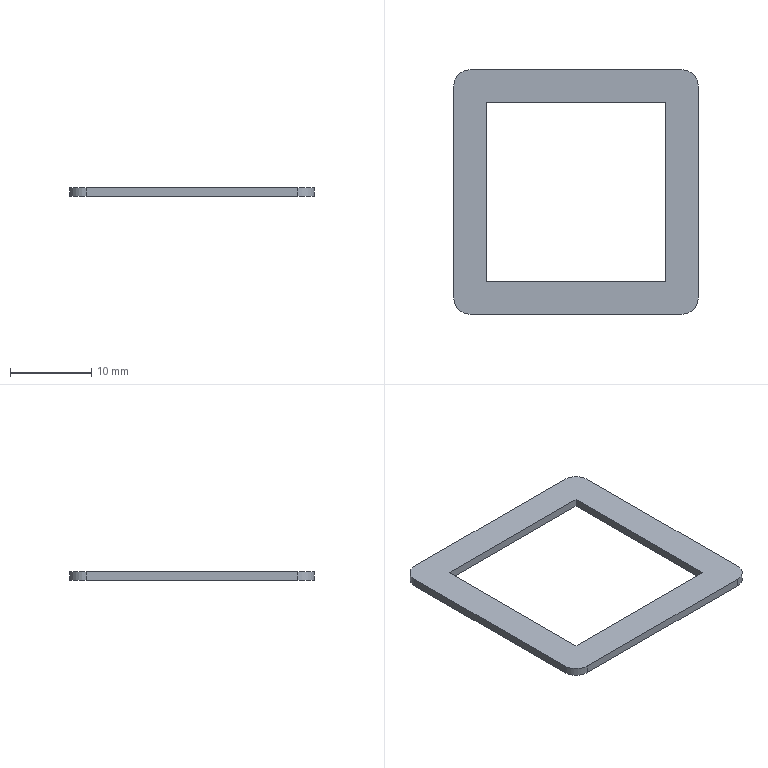Part | STEP file | 1 solid | 14 faces | box 30 x 30 x 1 mm | volume 412.566 mm3 | plane 10 | cylinder 4 | commonest cylinder face diameters 4 x4
STEP:
#1=CARTESIAN_POINT('',(0.,0.,0.));
#2=DIRECTION('',(0.,0.,1.));
#3=DIRECTION('',(1.,0.,0.));
#4=AXIS2_PLACEMENT_3D('',#1,#2,#3);
#5=CARTESIAN_POINT('',(13.,15.,1.));
#6=VERTEX_POINT('',#5);
#7=CARTESIAN_POINT('',(-13.,15.,1.));
#8=VERTEX_POINT('',#7);
#9=CARTESIAN_POINT('',(15.,15.,1.));
#10=DIRECTION('',(-1.,0.,0.));
#11=VECTOR('',#10,1.);
#12=LINE('',#9,#11);
#13=CARTESIAN_POINT('',(0.,0.,1.));
#14=DIRECTION('',(0.,0.,-1.));
#15=DIRECTION('',(-1.,0.,0.));
#16=AXIS2_PLACEMENT_3D('',#13,#14,#15);
#17=PLANE('',#16);
#18=CARTESIAN_POINT('',(-15.,15.));
#19=DIRECTION('',(1.,0.));
#20=VECTOR('',#19,1.);
#21=LINE('',#18,#20);
#22=(GEOMETRIC_REPRESENTATION_CONTEXT(2)PARAMETRIC_REPRESENTATION_CONTEXT()REPRESENTATION_CONTEXT('',''));
#23=DEFINITIONAL_REPRESENTATION('',(#21),#22);
#24=PCURVE('',#17,#23);
#25=CARTESIAN_POINT('',(15.,15.,1.));
#26=DIRECTION('',(0.,-1.,0.));
#27=DIRECTION('',(0.,0.,-1.));
#28=AXIS2_PLACEMENT_3D('',#25,#26,#27);
#29=PLANE('',#28);
#30=CARTESIAN_POINT('',(0.,0.));
#31=DIRECTION('',(0.,-1.));
#32=VECTOR('',#31,1.);
#33=LINE('',#30,#32);
#34=(GEOMETRIC_REPRESENTATION_CONTEXT(2)PARAMETRIC_REPRESENTATION_CONTEXT()REPRESENTATION_CONTEXT('',''));
#35=DEFINITIONAL_REPRESENTATION('',(#33),#34);
#36=PCURVE('',#29,#35);
#37=SURFACE_CURVE('',#12,(#24,#36),.PCURVE_S1.);
#38=EDGE_CURVE('',#6,#8,#37,.T.);
#39=ORIENTED_EDGE('',*,*,#38,.T.);
#40=CARTESIAN_POINT('',(-15.,13.,1.));
#41=VERTEX_POINT('',#40);
#42=CARTESIAN_POINT('',(-13.,13.,1.));
#43=DIRECTION('',(0.,0.,1.));
#44=DIRECTION('',(-1.,0.,0.));
#45=AXIS2_PLACEMENT_3D('',#42,#43,#44);
#46=CIRCLE('',#45,2.);
#47=CARTESIAN_POINT('',(15.,13.));
#48=CARTESIAN_POINT('',(15.,9.536));
#49=CARTESIAN_POINT('',(12.,11.268));
#50=CARTESIAN_POINT('',(9.,13.));
#51=CARTESIAN_POINT('',(12.,14.732));
#52=CARTESIAN_POINT('',(15.,16.464));
#53=CARTESIAN_POINT('',(15.,13.));
#54=(BOUNDED_CURVE()B_SPLINE_CURVE(2,(#47,#48,#49,#50,#51,#52,#53),.UNSPECIFIED.,.T.,.F.)B_SPLINE_CURVE_WITH_KNOTS((1,2,2,2,2,1),(-2.094,0.,2.094,4.189,6.283,8.378),.UNSPECIFIED.)CURVE()GEOMETRIC_REPRESENTATION_ITEM()RATIONAL_B_SPLINE_CURVE((1.,0.5,1.,0.5,1.,0.5,1.))REPRESENTATION_ITEM(''));
#55=(GEOMETRIC_REPRESENTATION_CONTEXT(2)PARAMETRIC_REPRESENTATION_CONTEXT()REPRESENTATION_CONTEXT('',''));
#56=DEFINITIONAL_REPRESENTATION('',(#54),#55);
#57=PCURVE('',#17,#56);
#58=CARTESIAN_POINT('',(-13.,13.,1.));
#59=DIRECTION('',(0.,0.,-1.));
#60=DIRECTION('',(-1.,0.,0.));
#61=AXIS2_PLACEMENT_3D('',#58,#59,#60);
#62=CYLINDRICAL_SURFACE('',#61,2.);
#63=CARTESIAN_POINT('',(6.283,0.));
#64=DIRECTION('',(-1.,0.));
#65=VECTOR('',#64,1.);
#66=LINE('',#63,#65);
#67=(GEOMETRIC_REPRESENTATION_CONTEXT(2)PARAMETRIC_REPRESENTATION_CONTEXT()REPRESENTATION_CONTEXT('',''));
#68=DEFINITIONAL_REPRESENTATION('',(#66),#67);
#69=PCURVE('',#62,#68);
#70=SURFACE_CURVE('',#46,(#57,#69),.PCURVE_S1.);
#71=EDGE_CURVE('',#8,#41,#70,.T.);
#72=ORIENTED_EDGE('',*,*,#71,.T.);
#73=CARTESIAN_POINT('',(-15.,-13.,1.));
#74=VERTEX_POINT('',#73);
#75=CARTESIAN_POINT('',(-15.,15.,1.));
#76=DIRECTION('',(0.,-1.,0.));
#77=VECTOR('',#76,1.);
#78=LINE('',#75,#77);
#79=CARTESIAN_POINT('',(15.,15.));
#80=DIRECTION('',(0.,-1.));
#81=VECTOR('',#80,1.);
#82=LINE('',#79,#81);
#83=(GEOMETRIC_REPRESENTATION_CONTEXT(2)PARAMETRIC_REPRESENTATION_CONTEXT()REPRESENTATION_CONTEXT('',''));
#84=DEFINITIONAL_REPRESENTATION('',(#82),#83);
#85=PCURVE('',#17,#84);
#86=CARTESIAN_POINT('',(-15.,15.,1.));
#87=DIRECTION('',(1.,0.,0.));
#88=DIRECTION('',(0.,0.,-1.));
#89=AXIS2_PLACEMENT_3D('',#86,#87,#88);
#90=PLANE('',#89);
#91=CARTESIAN_POINT('',(0.,0.));
#92=DIRECTION('',(0.,-1.));
#93=VECTOR('',#92,1.);
#94=LINE('',#91,#93);
#95=(GEOMETRIC_REPRESENTATION_CONTEXT(2)PARAMETRIC_REPRESENTATION_CONTEXT()REPRESENTATION_CONTEXT('',''));
#96=DEFINITIONAL_REPRESENTATION('',(#94),#95);
#97=PCURVE('',#90,#96);
#98=SURFACE_CURVE('',#78,(#85,#97),.PCURVE_S1.);
#99=EDGE_CURVE('',#41,#74,#98,.T.);
#100=ORIENTED_EDGE('',*,*,#99,.T.);
#101=CARTESIAN_POINT('',(-13.,-15.,1.));
#102=VERTEX_POINT('',#101);
#103=CARTESIAN_POINT('',(-13.,-13.,1.));
#104=DIRECTION('',(0.,0.,1.));
#105=DIRECTION('',(-1.,0.,0.));
#106=AXIS2_PLACEMENT_3D('',#103,#104,#105);
#107=CIRCLE('',#106,2.);
#108=CARTESIAN_POINT('',(15.,-13.));
#109=CARTESIAN_POINT('',(15.,-16.464));
#110=CARTESIAN_POINT('',(12.,-14.732));
#111=CARTESIAN_POINT('',(9.,-13.));
#112=CARTESIAN_POINT('',(12.,-11.268));
#113=CARTESIAN_POINT('',(15.,-9.536));
#114=CARTESIAN_POINT('',(15.,-13.));
#115=(BOUNDED_CURVE()B_SPLINE_CURVE(2,(#108,#109,#110,#111,#112,#113,#114),.UNSPECIFIED.,.T.,.F.)B_SPLINE_CURVE_WITH_KNOTS((1,2,2,2,2,1),(-2.094,0.,2.094,4.189,6.283,8.378),.UNSPECIFIED.)CURVE()GEOMETRIC_REPRESENTATION_ITEM()RATIONAL_B_SPLINE_CURVE((1.,0.5,1.,0.5,1.,0.5,1.))REPRESENTATION_ITEM(''));
#116=(GEOMETRIC_REPRESENTATION_CONTEXT(2)PARAMETRIC_REPRESENTATION_CONTEXT()REPRESENTATION_CONTEXT('',''));
#117=DEFINITIONAL_REPRESENTATION('',(#115),#116);
#118=PCURVE('',#17,#117);
#119=CARTESIAN_POINT('',(-13.,-13.,1.));
#120=DIRECTION('',(0.,0.,-1.));
#121=DIRECTION('',(-1.,0.,0.));
#122=AXIS2_PLACEMENT_3D('',#119,#120,#121);
#123=CYLINDRICAL_SURFACE('',#122,2.);
#124=CARTESIAN_POINT('',(6.283,0.));
#125=DIRECTION('',(-1.,0.));
#126=VECTOR('',#125,1.);
#127=LINE('',#124,#126);
#128=(GEOMETRIC_REPRESENTATION_CONTEXT(2)PARAMETRIC_REPRESENTATION_CONTEXT()REPRESENTATION_CONTEXT('',''));
#129=DEFINITIONAL_REPRESENTATION('',(#127),#128);
#130=PCURVE('',#123,#129);
#131=SURFACE_CURVE('',#107,(#118,#130),.PCURVE_S1.);
#132=EDGE_CURVE('',#74,#102,#131,.T.);
#133=ORIENTED_EDGE('',*,*,#132,.T.);
#134=CARTESIAN_POINT('',(13.,-15.,1.));
#135=VERTEX_POINT('',#134);
#136=CARTESIAN_POINT('',(15.,-15.,1.));
#137=DIRECTION('',(1.,0.,0.));
#138=VECTOR('',#137,1.);
#139=LINE('',#136,#138);
#140=CARTESIAN_POINT('',(-15.,-15.));
#141=DIRECTION('',(-1.,0.));
#142=VECTOR('',#141,1.);
#143=LINE('',#140,#142);
#144=(GEOMETRIC_REPRESENTATION_CONTEXT(2)PARAMETRIC_REPRESENTATION_CONTEXT()REPRESENTATION_CONTEXT('',''));
#145=DEFINITIONAL_REPRESENTATION('',(#143),#144);
#146=PCURVE('',#17,#145);
#147=CARTESIAN_POINT('',(15.,-15.,1.));
#148=DIRECTION('',(0.,1.,0.));
#149=DIRECTION('',(0.,0.,1.));
#150=AXIS2_PLACEMENT_3D('',#147,#148,#149);
#151=PLANE('',#150);
#152=CARTESIAN_POINT('',(0.,0.));
#153=DIRECTION('',(0.,1.));
#154=VECTOR('',#153,1.);
#155=LINE('',#152,#154);
#156=(GEOMETRIC_REPRESENTATION_CONTEXT(2)PARAMETRIC_REPRESENTATION_CONTEXT()REPRESENTATION_CONTEXT('',''));
#157=DEFINITIONAL_REPRESENTATION('',(#155),#156);
#158=PCURVE('',#151,#157);
#159=SURFACE_CURVE('',#139,(#146,#158),.PCURVE_S1.);
#160=EDGE_CURVE('',#102,#135,#159,.T.);
#161=ORIENTED_EDGE('',*,*,#160,.T.);
#162=CARTESIAN_POINT('',(15.,-13.,1.));
#163=VERTEX_POINT('',#162);
#164=CARTESIAN_POINT('',(13.,-13.,1.));
#165=DIRECTION('',(0.,0.,1.));
#166=DIRECTION('',(-1.,0.,0.));
#167=AXIS2_PLACEMENT_3D('',#164,#165,#166);
#168=CIRCLE('',#167,2.);
#169=CARTESIAN_POINT('',(-11.,-13.));
#170=CARTESIAN_POINT('',(-11.,-16.464));
#171=CARTESIAN_POINT('',(-14.,-14.732));
#172=CARTESIAN_POINT('',(-17.,-13.));
#173=CARTESIAN_POINT('',(-14.,-11.268));
#174=CARTESIAN_POINT('',(-11.,-9.536));
#175=CARTESIAN_POINT('',(-11.,-13.));
#176=(BOUNDED_CURVE()B_SPLINE_CURVE(2,(#169,#170,#171,#172,#173,#174,#175),.UNSPECIFIED.,.T.,.F.)B_SPLINE_CURVE_WITH_KNOTS((1,2,2,2,2,1),(-2.094,0.,2.094,4.189,6.283,8.378),.UNSPECIFIED.)CURVE()GEOMETRIC_REPRESENTATION_ITEM()RATIONAL_B_SPLINE_CURVE((1.,0.5,1.,0.5,1.,0.5,1.))REPRESENTATION_ITEM(''));
#177=(GEOMETRIC_REPRESENTATION_CONTEXT(2)PARAMETRIC_REPRESENTATION_CONTEXT()REPRESENTATION_CONTEXT('',''));
#178=DEFINITIONAL_REPRESENTATION('',(#176),#177);
#179=PCURVE('',#17,#178);
#180=CARTESIAN_POINT('',(13.,-13.,1.));
#181=DIRECTION('',(0.,0.,-1.));
#182=DIRECTION('',(-1.,0.,0.));
#183=AXIS2_PLACEMENT_3D('',#180,#181,#182);
#184=CYLINDRICAL_SURFACE('',#183,2.);
#185=CARTESIAN_POINT('',(6.283,0.));
#186=DIRECTION('',(-1.,0.));
#187=VECTOR('',#186,1.);
#188=LINE('',#185,#187);
#189=(GEOMETRIC_REPRESENTATION_CONTEXT(2)PARAMETRIC_REPRESENTATION_CONTEXT()REPRESENTATION_CONTEXT('',''));
#190=DEFINITIONAL_REPRESENTATION('',(#188),#189);
#191=PCURVE('',#184,#190);
#192=SURFACE_CURVE('',#168,(#179,#191),.PCURVE_S1.);
#193=EDGE_CURVE('',#135,#163,#192,.T.);
#194=ORIENTED_EDGE('',*,*,#193,.T.);
#195=CARTESIAN_POINT('',(15.,13.,1.));
#196=VERTEX_POINT('',#195);
#197=CARTESIAN_POINT('',(15.,15.,1.));
#198=DIRECTION('',(0.,1.,0.));
#199=VECTOR('',#198,1.);
#200=LINE('',#197,#199);
#201=CARTESIAN_POINT('',(-15.,15.));
#202=DIRECTION('',(0.,1.));
#203=VECTOR('',#202,1.);
#204=LINE('',#201,#203);
#205=(GEOMETRIC_REPRESENTATION_CONTEXT(2)PARAMETRIC_REPRESENTATION_CONTEXT()REPRESENTATION_CONTEXT('',''));
#206=DEFINITIONAL_REPRESENTATION('',(#204),#205);
#207=PCURVE('',#17,#206);
#208=CARTESIAN_POINT('',(15.,15.,1.));
#209=DIRECTION('',(-1.,0.,0.));
#210=DIRECTION('',(0.,0.,1.));
#211=AXIS2_PLACEMENT_3D('',#208,#209,#210);
#212=PLANE('',#211);
#213=CARTESIAN_POINT('',(0.,0.));
#214=DIRECTION('',(0.,1.));
#215=VECTOR('',#214,1.);
#216=LINE('',#213,#215);
#217=(GEOMETRIC_REPRESENTATION_CONTEXT(2)PARAMETRIC_REPRESENTATION_CONTEXT()REPRESENTATION_CONTEXT('',''));
#218=DEFINITIONAL_REPRESENTATION('',(#216),#217);
#219=PCURVE('',#212,#218);
#220=SURFACE_CURVE('',#200,(#207,#219),.PCURVE_S1.);
#221=EDGE_CURVE('',#163,#196,#220,.T.);
#222=ORIENTED_EDGE('',*,*,#221,.T.);
#223=CARTESIAN_POINT('',(13.,13.,1.));
#224=DIRECTION('',(0.,0.,1.));
#225=DIRECTION('',(-1.,0.,0.));
#226=AXIS2_PLACEMENT_3D('',#223,#224,#225);
#227=CIRCLE('',#226,2.);
#228=CARTESIAN_POINT('',(-11.,13.));
#229=CARTESIAN_POINT('',(-11.,9.536));
#230=CARTESIAN_POINT('',(-14.,11.268));
#231=CARTESIAN_POINT('',(-17.,13.));
#232=CARTESIAN_POINT('',(-14.,14.732));
#233=CARTESIAN_POINT('',(-11.,16.464));
#234=CARTESIAN_POINT('',(-11.,13.));
#235=(BOUNDED_CURVE()B_SPLINE_CURVE(2,(#228,#229,#230,#231,#232,#233,#234),.UNSPECIFIED.,.T.,.F.)B_SPLINE_CURVE_WITH_KNOTS((1,2,2,2,2,1),(-2.094,0.,2.094,4.189,6.283,8.378),.UNSPECIFIED.)CURVE()GEOMETRIC_REPRESENTATION_ITEM()RATIONAL_B_SPLINE_CURVE((1.,0.5,1.,0.5,1.,0.5,1.))REPRESENTATION_ITEM(''));
#236=(GEOMETRIC_REPRESENTATION_CONTEXT(2)PARAMETRIC_REPRESENTATION_CONTEXT()REPRESENTATION_CONTEXT('',''));
#237=DEFINITIONAL_REPRESENTATION('',(#235),#236);
#238=PCURVE('',#17,#237);
#239=CARTESIAN_POINT('',(13.,13.,1.));
#240=DIRECTION('',(0.,0.,-1.));
#241=DIRECTION('',(-1.,0.,0.));
#242=AXIS2_PLACEMENT_3D('',#239,#240,#241);
#243=CYLINDRICAL_SURFACE('',#242,2.);
#244=CARTESIAN_POINT('',(6.283,0.));
#245=DIRECTION('',(-1.,0.));
#246=VECTOR('',#245,1.);
#247=LINE('',#244,#246);
#248=(GEOMETRIC_REPRESENTATION_CONTEXT(2)PARAMETRIC_REPRESENTATION_CONTEXT()REPRESENTATION_CONTEXT('',''));
#249=DEFINITIONAL_REPRESENTATION('',(#247),#248);
#250=PCURVE('',#243,#249);
#251=SURFACE_CURVE('',#227,(#238,#250),.PCURVE_S1.);
#252=EDGE_CURVE('',#196,#6,#251,.T.);
#253=ORIENTED_EDGE('',*,*,#252,.T.);
#254=EDGE_LOOP('',(#39,#72,#100,#133,#161,#194,#222,#253));
#255=FACE_BOUND('',#254,.T.);
#256=CARTESIAN_POINT('',(-11.,11.,1.));
#257=VERTEX_POINT('',#256);
#258=CARTESIAN_POINT('',(-11.,-11.,1.));
#259=VERTEX_POINT('',#258);
#260=CARTESIAN_POINT('',(-11.,11.,1.));
#261=DIRECTION('',(0.,-1.,0.));
#262=VECTOR('',#261,1.);
#263=LINE('',#260,#262);
#264=CARTESIAN_POINT('',(11.,11.));
#265=DIRECTION('',(0.,-1.));
#266=VECTOR('',#265,1.);
#267=LINE('',#264,#266);
#268=(GEOMETRIC_REPRESENTATION_CONTEXT(2)PARAMETRIC_REPRESENTATION_CONTEXT()REPRESENTATION_CONTEXT('',''));
#269=DEFINITIONAL_REPRESENTATION('',(#267),#268);
#270=PCURVE('',#17,#269);
#271=CARTESIAN_POINT('',(-11.,11.,1.));
#272=DIRECTION('',(1.,0.,0.));
#273=DIRECTION('',(0.,1.,0.));
#274=AXIS2_PLACEMENT_3D('',#271,#272,#273);
#275=PLANE('',#274);
#276=CARTESIAN_POINT('',(0.,0.));
#277=DIRECTION('',(-1.,0.));
#278=VECTOR('',#277,1.);
#279=LINE('',#276,#278);
#280=(GEOMETRIC_REPRESENTATION_CONTEXT(2)PARAMETRIC_REPRESENTATION_CONTEXT()REPRESENTATION_CONTEXT('',''));
#281=DEFINITIONAL_REPRESENTATION('',(#279),#280);
#282=PCURVE('',#275,#281);
#283=SURFACE_CURVE('',#263,(#270,#282),.PCURVE_S1.);
#284=EDGE_CURVE('',#257,#259,#283,.T.);
#285=ORIENTED_EDGE('',*,*,#284,.F.);
#286=CARTESIAN_POINT('',(11.,11.,1.));
#287=VERTEX_POINT('',#286);
#288=CARTESIAN_POINT('',(11.,11.,1.));
#289=DIRECTION('',(-1.,0.,0.));
#290=VECTOR('',#289,1.);
#291=LINE('',#288,#290);
#292=CARTESIAN_POINT('',(-11.,11.));
#293=DIRECTION('',(1.,0.));
#294=VECTOR('',#293,1.);
#295=LINE('',#292,#294);
#296=(GEOMETRIC_REPRESENTATION_CONTEXT(2)PARAMETRIC_REPRESENTATION_CONTEXT()REPRESENTATION_CONTEXT('',''));
#297=DEFINITIONAL_REPRESENTATION('',(#295),#296);
#298=PCURVE('',#17,#297);
#299=CARTESIAN_POINT('',(11.,11.,1.));
#300=DIRECTION('',(0.,-1.,0.));
#301=DIRECTION('',(1.,0.,0.));
#302=AXIS2_PLACEMENT_3D('',#299,#300,#301);
#303=PLANE('',#302);
#304=CARTESIAN_POINT('',(0.,0.));
#305=DIRECTION('',(-1.,0.));
#306=VECTOR('',#305,1.);
#307=LINE('',#304,#306);
#308=(GEOMETRIC_REPRESENTATION_CONTEXT(2)PARAMETRIC_REPRESENTATION_CONTEXT()REPRESENTATION_CONTEXT('',''));
#309=DEFINITIONAL_REPRESENTATION('',(#307),#308);
#310=PCURVE('',#303,#309);
#311=SURFACE_CURVE('',#291,(#298,#310),.PCURVE_S1.);
#312=EDGE_CURVE('',#287,#257,#311,.T.);
#313=ORIENTED_EDGE('',*,*,#312,.F.);
#314=CARTESIAN_POINT('',(11.,-11.,1.));
#315=VERTEX_POINT('',#314);
#316=CARTESIAN_POINT('',(11.,11.,1.));
#317=DIRECTION('',(0.,1.,0.));
#318=VECTOR('',#317,1.);
#319=LINE('',#316,#318);
#320=CARTESIAN_POINT('',(-11.,11.));
#321=DIRECTION('',(0.,1.));
#322=VECTOR('',#321,1.);
#323=LINE('',#320,#322);
#324=(GEOMETRIC_REPRESENTATION_CONTEXT(2)PARAMETRIC_REPRESENTATION_CONTEXT()REPRESENTATION_CONTEXT('',''));
#325=DEFINITIONAL_REPRESENTATION('',(#323),#324);
#326=PCURVE('',#17,#325);
#327=CARTESIAN_POINT('',(11.,11.,1.));
#328=DIRECTION('',(-1.,0.,0.));
#329=DIRECTION('',(0.,-1.,0.));
#330=AXIS2_PLACEMENT_3D('',#327,#328,#329);
#331=PLANE('',#330);
#332=CARTESIAN_POINT('',(0.,0.));
#333=DIRECTION('',(-1.,0.));
#334=VECTOR('',#333,1.);
#335=LINE('',#332,#334);
#336=(GEOMETRIC_REPRESENTATION_CONTEXT(2)PARAMETRIC_REPRESENTATION_CONTEXT()REPRESENTATION_CONTEXT('',''));
#337=DEFINITIONAL_REPRESENTATION('',(#335),#336);
#338=PCURVE('',#331,#337);
#339=SURFACE_CURVE('',#319,(#326,#338),.PCURVE_S1.);
#340=EDGE_CURVE('',#315,#287,#339,.T.);
#341=ORIENTED_EDGE('',*,*,#340,.F.);
#342=CARTESIAN_POINT('',(11.,-11.,1.));
#343=DIRECTION('',(1.,0.,0.));
#344=VECTOR('',#343,1.);
#345=LINE('',#342,#344);
#346=CARTESIAN_POINT('',(-11.,-11.));
#347=DIRECTION('',(-1.,0.));
#348=VECTOR('',#347,1.);
#349=LINE('',#346,#348);
#350=(GEOMETRIC_REPRESENTATION_CONTEXT(2)PARAMETRIC_REPRESENTATION_CONTEXT()REPRESENTATION_CONTEXT('',''));
#351=DEFINITIONAL_REPRESENTATION('',(#349),#350);
#352=PCURVE('',#17,#351);
#353=CARTESIAN_POINT('',(11.,-11.,1.));
#354=DIRECTION('',(0.,1.,0.));
#355=DIRECTION('',(-1.,0.,0.));
#356=AXIS2_PLACEMENT_3D('',#353,#354,#355);
#357=PLANE('',#356);
#358=CARTESIAN_POINT('',(0.,0.));
#359=DIRECTION('',(-1.,0.));
#360=VECTOR('',#359,1.);
#361=LINE('',#358,#360);
#362=(GEOMETRIC_REPRESENTATION_CONTEXT(2)PARAMETRIC_REPRESENTATION_CONTEXT()REPRESENTATION_CONTEXT('',''));
#363=DEFINITIONAL_REPRESENTATION('',(#361),#362);
#364=PCURVE('',#357,#363);
#365=SURFACE_CURVE('',#345,(#352,#364),.PCURVE_S1.);
#366=EDGE_CURVE('',#259,#315,#365,.T.);
#367=ORIENTED_EDGE('',*,*,#366,.F.);
#368=EDGE_LOOP('',(#285,#313,#341,#367));
#369=FACE_BOUND('',#368,.T.);
#370=ADVANCED_FACE('',(#255,#369),#17,.F.);
#371=CARTESIAN_POINT('',(-15.,13.,0.));
#372=VERTEX_POINT('',#371);
#373=CARTESIAN_POINT('',(-15.,-13.,0.));
#374=VERTEX_POINT('',#373);
#375=CARTESIAN_POINT('',(-15.,15.,0.));
#376=DIRECTION('',(0.,-1.,0.));
#377=VECTOR('',#376,1.);
#378=LINE('',#375,#377);
#379=CARTESIAN_POINT('',(0.,0.,0.));
#380=DIRECTION('',(0.,0.,-1.));
#381=DIRECTION('',(-1.,0.,0.));
#382=AXIS2_PLACEMENT_3D('',#379,#380,#381);
#383=PLANE('',#382);
#384=CARTESIAN_POINT('',(15.,15.));
#385=DIRECTION('',(0.,-1.));
#386=VECTOR('',#385,1.);
#387=LINE('',#384,#386);
#388=(GEOMETRIC_REPRESENTATION_CONTEXT(2)PARAMETRIC_REPRESENTATION_CONTEXT()REPRESENTATION_CONTEXT('',''));
#389=DEFINITIONAL_REPRESENTATION('',(#387),#388);
#390=PCURVE('',#383,#389);
#391=CARTESIAN_POINT('',(1.,0.));
#392=DIRECTION('',(0.,-1.));
#393=VECTOR('',#392,1.);
#394=LINE('',#391,#393);
#395=(GEOMETRIC_REPRESENTATION_CONTEXT(2)PARAMETRIC_REPRESENTATION_CONTEXT()REPRESENTATION_CONTEXT('',''));
#396=DEFINITIONAL_REPRESENTATION('',(#394),#395);
#397=PCURVE('',#90,#396);
#398=SURFACE_CURVE('',#378,(#390,#397),.PCURVE_S1.);
#399=EDGE_CURVE('',#372,#374,#398,.T.);
#400=ORIENTED_EDGE('',*,*,#399,.F.);
#401=CARTESIAN_POINT('',(-13.,15.,0.));
#402=VERTEX_POINT('',#401);
#403=CARTESIAN_POINT('',(-13.,13.,0.));
#404=DIRECTION('',(0.,0.,-1.));
#405=DIRECTION('',(-1.,0.,0.));
#406=AXIS2_PLACEMENT_3D('',#403,#404,#405);
#407=CIRCLE('',#406,2.);
#408=CARTESIAN_POINT('',(13.,13.));
#409=DIRECTION('',(1.,0.));
#410=AXIS2_PLACEMENT_2D('',#408,#409);
#411=CIRCLE('',#410,2.);
#412=(GEOMETRIC_REPRESENTATION_CONTEXT(2)PARAMETRIC_REPRESENTATION_CONTEXT()REPRESENTATION_CONTEXT('',''));
#413=DEFINITIONAL_REPRESENTATION('',(#411),#412);
#414=PCURVE('',#383,#413);
#415=CARTESIAN_POINT('',(0.,1.));
#416=DIRECTION('',(1.,0.));
#417=VECTOR('',#416,1.);
#418=LINE('',#415,#417);
#419=(GEOMETRIC_REPRESENTATION_CONTEXT(2)PARAMETRIC_REPRESENTATION_CONTEXT()REPRESENTATION_CONTEXT('',''));
#420=DEFINITIONAL_REPRESENTATION('',(#418),#419);
#421=PCURVE('',#62,#420);
#422=SURFACE_CURVE('',#407,(#414,#421),.PCURVE_S1.);
#423=EDGE_CURVE('',#372,#402,#422,.T.);
#424=ORIENTED_EDGE('',*,*,#423,.T.);
#425=CARTESIAN_POINT('',(13.,15.,0.));
#426=VERTEX_POINT('',#425);
#427=CARTESIAN_POINT('',(15.,15.,0.));
#428=DIRECTION('',(-1.,0.,0.));
#429=VECTOR('',#428,1.);
#430=LINE('',#427,#429);
#431=CARTESIAN_POINT('',(-15.,15.));
#432=DIRECTION('',(1.,0.));
#433=VECTOR('',#432,1.);
#434=LINE('',#431,#433);
#435=(GEOMETRIC_REPRESENTATION_CONTEXT(2)PARAMETRIC_REPRESENTATION_CONTEXT()REPRESENTATION_CONTEXT('',''));
#436=DEFINITIONAL_REPRESENTATION('',(#434),#435);
#437=PCURVE('',#383,#436);
#438=CARTESIAN_POINT('',(1.,0.));
#439=DIRECTION('',(0.,-1.));
#440=VECTOR('',#439,1.);
#441=LINE('',#438,#440);
#442=(GEOMETRIC_REPRESENTATION_CONTEXT(2)PARAMETRIC_REPRESENTATION_CONTEXT()REPRESENTATION_CONTEXT('',''));
#443=DEFINITIONAL_REPRESENTATION('',(#441),#442);
#444=PCURVE('',#29,#443);
#445=SURFACE_CURVE('',#430,(#437,#444),.PCURVE_S1.);
#446=EDGE_CURVE('',#426,#402,#445,.T.);
#447=ORIENTED_EDGE('',*,*,#446,.F.);
#448=CARTESIAN_POINT('',(15.,13.,0.));
#449=VERTEX_POINT('',#448);
#450=CARTESIAN_POINT('',(13.,13.,0.));
#451=DIRECTION('',(0.,0.,-1.));
#452=DIRECTION('',(-1.,0.,0.));
#453=AXIS2_PLACEMENT_3D('',#450,#451,#452);
#454=CIRCLE('',#453,2.);
#455=CARTESIAN_POINT('',(-13.,13.));
#456=DIRECTION('',(1.,0.));
#457=AXIS2_PLACEMENT_2D('',#455,#456);
#458=CIRCLE('',#457,2.);
#459=(GEOMETRIC_REPRESENTATION_CONTEXT(2)PARAMETRIC_REPRESENTATION_CONTEXT()REPRESENTATION_CONTEXT('',''));
#460=DEFINITIONAL_REPRESENTATION('',(#458),#459);
#461=PCURVE('',#383,#460);
#462=CARTESIAN_POINT('',(0.,1.));
#463=DIRECTION('',(1.,0.));
#464=VECTOR('',#463,1.);
#465=LINE('',#462,#464);
#466=(GEOMETRIC_REPRESENTATION_CONTEXT(2)PARAMETRIC_REPRESENTATION_CONTEXT()REPRESENTATION_CONTEXT('',''));
#467=DEFINITIONAL_REPRESENTATION('',(#465),#466);
#468=PCURVE('',#243,#467);
#469=SURFACE_CURVE('',#454,(#461,#468),.PCURVE_S1.);
#470=EDGE_CURVE('',#426,#449,#469,.T.);
#471=ORIENTED_EDGE('',*,*,#470,.T.);
#472=CARTESIAN_POINT('',(15.,-13.,0.));
#473=VERTEX_POINT('',#472);
#474=CARTESIAN_POINT('',(15.,15.,0.));
#475=DIRECTION('',(0.,1.,0.));
#476=VECTOR('',#475,1.);
#477=LINE('',#474,#476);
#478=CARTESIAN_POINT('',(-15.,15.));
#479=DIRECTION('',(0.,1.));
#480=VECTOR('',#479,1.);
#481=LINE('',#478,#480);
#482=(GEOMETRIC_REPRESENTATION_CONTEXT(2)PARAMETRIC_REPRESENTATION_CONTEXT()REPRESENTATION_CONTEXT('',''));
#483=DEFINITIONAL_REPRESENTATION('',(#481),#482);
#484=PCURVE('',#383,#483);
#485=CARTESIAN_POINT('',(-1.,0.));
#486=DIRECTION('',(0.,1.));
#487=VECTOR('',#486,1.);
#488=LINE('',#485,#487);
#489=(GEOMETRIC_REPRESENTATION_CONTEXT(2)PARAMETRIC_REPRESENTATION_CONTEXT()REPRESENTATION_CONTEXT('',''));
#490=DEFINITIONAL_REPRESENTATION('',(#488),#489);
#491=PCURVE('',#212,#490);
#492=SURFACE_CURVE('',#477,(#484,#491),.PCURVE_S1.);
#493=EDGE_CURVE('',#473,#449,#492,.T.);
#494=ORIENTED_EDGE('',*,*,#493,.F.);
#495=CARTESIAN_POINT('',(13.,-15.,0.));
#496=VERTEX_POINT('',#495);
#497=CARTESIAN_POINT('',(13.,-13.,0.));
#498=DIRECTION('',(0.,0.,-1.));
#499=DIRECTION('',(-1.,0.,0.));
#500=AXIS2_PLACEMENT_3D('',#497,#498,#499);
#501=CIRCLE('',#500,2.);
#502=CARTESIAN_POINT('',(-13.,-13.));
#503=DIRECTION('',(1.,0.));
#504=AXIS2_PLACEMENT_2D('',#502,#503);
#505=CIRCLE('',#504,2.);
#506=(GEOMETRIC_REPRESENTATION_CONTEXT(2)PARAMETRIC_REPRESENTATION_CONTEXT()REPRESENTATION_CONTEXT('',''));
#507=DEFINITIONAL_REPRESENTATION('',(#505),#506);
#508=PCURVE('',#383,#507);
#509=CARTESIAN_POINT('',(0.,1.));
#510=DIRECTION('',(1.,0.));
#511=VECTOR('',#510,1.);
#512=LINE('',#509,#511);
#513=(GEOMETRIC_REPRESENTATION_CONTEXT(2)PARAMETRIC_REPRESENTATION_CONTEXT()REPRESENTATION_CONTEXT('',''));
#514=DEFINITIONAL_REPRESENTATION('',(#512),#513);
#515=PCURVE('',#184,#514);
#516=SURFACE_CURVE('',#501,(#508,#515),.PCURVE_S1.);
#517=EDGE_CURVE('',#473,#496,#516,.T.);
#518=ORIENTED_EDGE('',*,*,#517,.T.);
#519=CARTESIAN_POINT('',(-13.,-15.,0.));
#520=VERTEX_POINT('',#519);
#521=CARTESIAN_POINT('',(15.,-15.,0.));
#522=DIRECTION('',(1.,0.,0.));
#523=VECTOR('',#522,1.);
#524=LINE('',#521,#523);
#525=CARTESIAN_POINT('',(-15.,-15.));
#526=DIRECTION('',(-1.,0.));
#527=VECTOR('',#526,1.);
#528=LINE('',#525,#527);
#529=(GEOMETRIC_REPRESENTATION_CONTEXT(2)PARAMETRIC_REPRESENTATION_CONTEXT()REPRESENTATION_CONTEXT('',''));
#530=DEFINITIONAL_REPRESENTATION('',(#528),#529);
#531=PCURVE('',#383,#530);
#532=CARTESIAN_POINT('',(-1.,0.));
#533=DIRECTION('',(0.,1.));
#534=VECTOR('',#533,1.);
#535=LINE('',#532,#534);
#536=(GEOMETRIC_REPRESENTATION_CONTEXT(2)PARAMETRIC_REPRESENTATION_CONTEXT()REPRESENTATION_CONTEXT('',''));
#537=DEFINITIONAL_REPRESENTATION('',(#535),#536);
#538=PCURVE('',#151,#537);
#539=SURFACE_CURVE('',#524,(#531,#538),.PCURVE_S1.);
#540=EDGE_CURVE('',#520,#496,#539,.T.);
#541=ORIENTED_EDGE('',*,*,#540,.F.);
#542=CARTESIAN_POINT('',(-13.,-13.,0.));
#543=DIRECTION('',(0.,0.,-1.));
#544=DIRECTION('',(-1.,0.,0.));
#545=AXIS2_PLACEMENT_3D('',#542,#543,#544);
#546=CIRCLE('',#545,2.);
#547=CARTESIAN_POINT('',(13.,-13.));
#548=DIRECTION('',(1.,0.));
#549=AXIS2_PLACEMENT_2D('',#547,#548);
#550=CIRCLE('',#549,2.);
#551=(GEOMETRIC_REPRESENTATION_CONTEXT(2)PARAMETRIC_REPRESENTATION_CONTEXT()REPRESENTATION_CONTEXT('',''));
#552=DEFINITIONAL_REPRESENTATION('',(#550),#551);
#553=PCURVE('',#383,#552);
#554=CARTESIAN_POINT('',(0.,1.));
#555=DIRECTION('',(1.,0.));
#556=VECTOR('',#555,1.);
#557=LINE('',#554,#556);
#558=(GEOMETRIC_REPRESENTATION_CONTEXT(2)PARAMETRIC_REPRESENTATION_CONTEXT()REPRESENTATION_CONTEXT('',''));
#559=DEFINITIONAL_REPRESENTATION('',(#557),#558);
#560=PCURVE('',#123,#559);
#561=SURFACE_CURVE('',#546,(#553,#560),.PCURVE_S1.);
#562=EDGE_CURVE('',#520,#374,#561,.T.);
#563=ORIENTED_EDGE('',*,*,#562,.T.);
#564=EDGE_LOOP('',(#400,#424,#447,#471,#494,#518,#541,#563));
#565=FACE_BOUND('',#564,.T.);
#566=CARTESIAN_POINT('',(11.,11.,0.));
#567=VERTEX_POINT('',#566);
#568=CARTESIAN_POINT('',(-11.,11.,0.));
#569=VERTEX_POINT('',#568);
#570=CARTESIAN_POINT('',(11.,11.,0.));
#571=DIRECTION('',(-1.,0.,0.));
#572=VECTOR('',#571,1.);
#573=LINE('',#570,#572);
#574=CARTESIAN_POINT('',(-11.,11.));
#575=DIRECTION('',(1.,0.));
#576=VECTOR('',#575,1.);
#577=LINE('',#574,#576);
#578=(GEOMETRIC_REPRESENTATION_CONTEXT(2)PARAMETRIC_REPRESENTATION_CONTEXT()REPRESENTATION_CONTEXT('',''));
#579=DEFINITIONAL_REPRESENTATION('',(#577),#578);
#580=PCURVE('',#383,#579);
#581=CARTESIAN_POINT('',(0.,-1.));
#582=DIRECTION('',(-1.,0.));
#583=VECTOR('',#582,1.);
#584=LINE('',#581,#583);
#585=(GEOMETRIC_REPRESENTATION_CONTEXT(2)PARAMETRIC_REPRESENTATION_CONTEXT()REPRESENTATION_CONTEXT('',''));
#586=DEFINITIONAL_REPRESENTATION('',(#584),#585);
#587=PCURVE('',#303,#586);
#588=SURFACE_CURVE('',#573,(#580,#587),.PCURVE_S1.);
#589=EDGE_CURVE('',#567,#569,#588,.T.);
#590=ORIENTED_EDGE('',*,*,#589,.T.);
#591=CARTESIAN_POINT('',(-11.,-11.,0.));
#592=VERTEX_POINT('',#591);
#593=CARTESIAN_POINT('',(-11.,11.,0.));
#594=DIRECTION('',(0.,-1.,0.));
#595=VECTOR('',#594,1.);
#596=LINE('',#593,#595);
#597=CARTESIAN_POINT('',(11.,11.));
#598=DIRECTION('',(0.,-1.));
#599=VECTOR('',#598,1.);
#600=LINE('',#597,#599);
#601=(GEOMETRIC_REPRESENTATION_CONTEXT(2)PARAMETRIC_REPRESENTATION_CONTEXT()REPRESENTATION_CONTEXT('',''));
#602=DEFINITIONAL_REPRESENTATION('',(#600),#601);
#603=PCURVE('',#383,#602);
#604=CARTESIAN_POINT('',(0.,-1.));
#605=DIRECTION('',(-1.,0.));
#606=VECTOR('',#605,1.);
#607=LINE('',#604,#606);
#608=(GEOMETRIC_REPRESENTATION_CONTEXT(2)PARAMETRIC_REPRESENTATION_CONTEXT()REPRESENTATION_CONTEXT('',''));
#609=DEFINITIONAL_REPRESENTATION('',(#607),#608);
#610=PCURVE('',#275,#609);
#611=SURFACE_CURVE('',#596,(#603,#610),.PCURVE_S1.);
#612=EDGE_CURVE('',#569,#592,#611,.T.);
#613=ORIENTED_EDGE('',*,*,#612,.T.);
#614=CARTESIAN_POINT('',(11.,-11.,0.));
#615=VERTEX_POINT('',#614);
#616=CARTESIAN_POINT('',(11.,-11.,0.));
#617=DIRECTION('',(1.,0.,0.));
#618=VECTOR('',#617,1.);
#619=LINE('',#616,#618);
#620=CARTESIAN_POINT('',(-11.,-11.));
#621=DIRECTION('',(-1.,0.));
#622=VECTOR('',#621,1.);
#623=LINE('',#620,#622);
#624=(GEOMETRIC_REPRESENTATION_CONTEXT(2)PARAMETRIC_REPRESENTATION_CONTEXT()REPRESENTATION_CONTEXT('',''));
#625=DEFINITIONAL_REPRESENTATION('',(#623),#624);
#626=PCURVE('',#383,#625);
#627=CARTESIAN_POINT('',(0.,-1.));
#628=DIRECTION('',(-1.,0.));
#629=VECTOR('',#628,1.);
#630=LINE('',#627,#629);
#631=(GEOMETRIC_REPRESENTATION_CONTEXT(2)PARAMETRIC_REPRESENTATION_CONTEXT()REPRESENTATION_CONTEXT('',''));
#632=DEFINITIONAL_REPRESENTATION('',(#630),#631);
#633=PCURVE('',#357,#632);
#634=SURFACE_CURVE('',#619,(#626,#633),.PCURVE_S1.);
#635=EDGE_CURVE('',#592,#615,#634,.T.);
#636=ORIENTED_EDGE('',*,*,#635,.T.);
#637=CARTESIAN_POINT('',(11.,11.,0.));
#638=DIRECTION('',(0.,1.,0.));
#639=VECTOR('',#638,1.);
#640=LINE('',#637,#639);
#641=CARTESIAN_POINT('',(-11.,11.));
#642=DIRECTION('',(0.,1.));
#643=VECTOR('',#642,1.);
#644=LINE('',#641,#643);
#645=(GEOMETRIC_REPRESENTATION_CONTEXT(2)PARAMETRIC_REPRESENTATION_CONTEXT()REPRESENTATION_CONTEXT('',''));
#646=DEFINITIONAL_REPRESENTATION('',(#644),#645);
#647=PCURVE('',#383,#646);
#648=CARTESIAN_POINT('',(0.,-1.));
#649=DIRECTION('',(-1.,0.));
#650=VECTOR('',#649,1.);
#651=LINE('',#648,#650);
#652=(GEOMETRIC_REPRESENTATION_CONTEXT(2)PARAMETRIC_REPRESENTATION_CONTEXT()REPRESENTATION_CONTEXT('',''));
#653=DEFINITIONAL_REPRESENTATION('',(#651),#652);
#654=PCURVE('',#331,#653);
#655=SURFACE_CURVE('',#640,(#647,#654),.PCURVE_S1.);
#656=EDGE_CURVE('',#615,#567,#655,.T.);
#657=ORIENTED_EDGE('',*,*,#656,.T.);
#658=EDGE_LOOP('',(#590,#613,#636,#657));
#659=FACE_BOUND('',#658,.T.);
#660=ADVANCED_FACE('',(#565,#659),#383,.T.);
#661=ORIENTED_EDGE('',*,*,#99,.F.);
#662=CARTESIAN_POINT('',(-15.,13.,1.));
#663=DIRECTION('',(0.,0.,-1.));
#664=VECTOR('',#663,1.);
#665=LINE('',#662,#664);
#666=CARTESIAN_POINT('',(0.,-2.));
#667=DIRECTION('',(1.,0.));
#668=VECTOR('',#667,1.);
#669=LINE('',#666,#668);
#670=(GEOMETRIC_REPRESENTATION_CONTEXT(2)PARAMETRIC_REPRESENTATION_CONTEXT()REPRESENTATION_CONTEXT('',''));
#671=DEFINITIONAL_REPRESENTATION('',(#669),#670);
#672=PCURVE('',#90,#671);
#673=CARTESIAN_POINT('',(0.,0.));
#674=DIRECTION('',(0.,1.));
#675=VECTOR('',#674,1.);
#676=LINE('',#673,#675);
#677=(GEOMETRIC_REPRESENTATION_CONTEXT(2)PARAMETRIC_REPRESENTATION_CONTEXT()REPRESENTATION_CONTEXT('',''));
#678=DEFINITIONAL_REPRESENTATION('',(#676),#677);
#679=PCURVE('',#62,#678);
#680=SURFACE_CURVE('',#665,(#672,#679),.PCURVE_S1.);
#681=EDGE_CURVE('',#41,#372,#680,.T.);
#682=ORIENTED_EDGE('',*,*,#681,.T.);
#683=ORIENTED_EDGE('',*,*,#399,.T.);
#684=CARTESIAN_POINT('',(-15.,-13.,1.));
#685=DIRECTION('',(0.,0.,1.));
#686=VECTOR('',#685,1.);
#687=LINE('',#684,#686);
#688=CARTESIAN_POINT('',(0.,-28.));
#689=DIRECTION('',(-1.,0.));
#690=VECTOR('',#689,1.);
#691=LINE('',#688,#690);
#692=(GEOMETRIC_REPRESENTATION_CONTEXT(2)PARAMETRIC_REPRESENTATION_CONTEXT()REPRESENTATION_CONTEXT('',''));
#693=DEFINITIONAL_REPRESENTATION('',(#691),#692);
#694=PCURVE('',#90,#693);
#695=CARTESIAN_POINT('',(6.283,0.));
#696=DIRECTION('',(0.,-1.));
#697=VECTOR('',#696,1.);
#698=LINE('',#695,#697);
#699=(GEOMETRIC_REPRESENTATION_CONTEXT(2)PARAMETRIC_REPRESENTATION_CONTEXT()REPRESENTATION_CONTEXT('',''));
#700=DEFINITIONAL_REPRESENTATION('',(#698),#699);
#701=PCURVE('',#123,#700);
#702=SURFACE_CURVE('',#687,(#694,#701),.PCURVE_S1.);
#703=EDGE_CURVE('',#374,#74,#702,.T.);
#704=ORIENTED_EDGE('',*,*,#703,.T.);
#705=EDGE_LOOP('',(#661,#682,#683,#704));
#706=FACE_BOUND('',#705,.T.);
#707=ADVANCED_FACE('',(#706),#90,.F.);
#708=ORIENTED_EDGE('',*,*,#540,.T.);
#709=CARTESIAN_POINT('',(13.,-15.,1.));
#710=DIRECTION('',(0.,0.,1.));
#711=VECTOR('',#710,1.);
#712=LINE('',#709,#711);
#713=CARTESIAN_POINT('',(0.,-2.));
#714=DIRECTION('',(1.,0.));
#715=VECTOR('',#714,1.);
#716=LINE('',#713,#715);
#717=(GEOMETRIC_REPRESENTATION_CONTEXT(2)PARAMETRIC_REPRESENTATION_CONTEXT()REPRESENTATION_CONTEXT('',''));
#718=DEFINITIONAL_REPRESENTATION('',(#716),#717);
#719=PCURVE('',#151,#718);
#720=CARTESIAN_POINT('',(4.712,0.));
#721=DIRECTION('',(0.,-1.));
#722=VECTOR('',#721,1.);
#723=LINE('',#720,#722);
#724=(GEOMETRIC_REPRESENTATION_CONTEXT(2)PARAMETRIC_REPRESENTATION_CONTEXT()REPRESENTATION_CONTEXT('',''));
#725=DEFINITIONAL_REPRESENTATION('',(#723),#724);
#726=PCURVE('',#184,#725);
#727=SURFACE_CURVE('',#712,(#719,#726),.PCURVE_S1.);
#728=EDGE_CURVE('',#496,#135,#727,.T.);
#729=ORIENTED_EDGE('',*,*,#728,.T.);
#730=ORIENTED_EDGE('',*,*,#160,.F.);
#731=CARTESIAN_POINT('',(-13.,-15.,1.));
#732=DIRECTION('',(0.,0.,-1.));
#733=VECTOR('',#732,1.);
#734=LINE('',#731,#733);
#735=CARTESIAN_POINT('',(0.,-28.));
#736=DIRECTION('',(-1.,0.));
#737=VECTOR('',#736,1.);
#738=LINE('',#735,#737);
#739=(GEOMETRIC_REPRESENTATION_CONTEXT(2)PARAMETRIC_REPRESENTATION_CONTEXT()REPRESENTATION_CONTEXT('',''));
#740=DEFINITIONAL_REPRESENTATION('',(#738),#739);
#741=PCURVE('',#151,#740);
#742=CARTESIAN_POINT('',(4.712,0.));
#743=DIRECTION('',(0.,1.));
#744=VECTOR('',#743,1.);
#745=LINE('',#742,#744);
#746=(GEOMETRIC_REPRESENTATION_CONTEXT(2)PARAMETRIC_REPRESENTATION_CONTEXT()REPRESENTATION_CONTEXT('',''));
#747=DEFINITIONAL_REPRESENTATION('',(#745),#746);
#748=PCURVE('',#123,#747);
#749=SURFACE_CURVE('',#734,(#741,#748),.PCURVE_S1.);
#750=EDGE_CURVE('',#102,#520,#749,.T.);
#751=ORIENTED_EDGE('',*,*,#750,.T.);
#752=EDGE_LOOP('',(#708,#729,#730,#751));
#753=FACE_BOUND('',#752,.T.);
#754=ADVANCED_FACE('',(#753),#151,.F.);
#755=ORIENTED_EDGE('',*,*,#493,.T.);
#756=CARTESIAN_POINT('',(15.,13.,1.));
#757=DIRECTION('',(0.,0.,1.));
#758=VECTOR('',#757,1.);
#759=LINE('',#756,#758);
#760=CARTESIAN_POINT('',(0.,-2.));
#761=DIRECTION('',(1.,0.));
#762=VECTOR('',#761,1.);
#763=LINE('',#760,#762);
#764=(GEOMETRIC_REPRESENTATION_CONTEXT(2)PARAMETRIC_REPRESENTATION_CONTEXT()REPRESENTATION_CONTEXT('',''));
#765=DEFINITIONAL_REPRESENTATION('',(#763),#764);
#766=PCURVE('',#212,#765);
#767=CARTESIAN_POINT('',(3.142,0.));
#768=DIRECTION('',(0.,-1.));
#769=VECTOR('',#768,1.);
#770=LINE('',#767,#769);
#771=(GEOMETRIC_REPRESENTATION_CONTEXT(2)PARAMETRIC_REPRESENTATION_CONTEXT()REPRESENTATION_CONTEXT('',''));
#772=DEFINITIONAL_REPRESENTATION('',(#770),#771);
#773=PCURVE('',#243,#772);
#774=SURFACE_CURVE('',#759,(#766,#773),.PCURVE_S1.);
#775=EDGE_CURVE('',#449,#196,#774,.T.);
#776=ORIENTED_EDGE('',*,*,#775,.T.);
#777=ORIENTED_EDGE('',*,*,#221,.F.);
#778=CARTESIAN_POINT('',(15.,-13.,1.));
#779=DIRECTION('',(0.,0.,-1.));
#780=VECTOR('',#779,1.);
#781=LINE('',#778,#780);
#782=CARTESIAN_POINT('',(0.,-28.));
#783=DIRECTION('',(-1.,0.));
#784=VECTOR('',#783,1.);
#785=LINE('',#782,#784);
#786=(GEOMETRIC_REPRESENTATION_CONTEXT(2)PARAMETRIC_REPRESENTATION_CONTEXT()REPRESENTATION_CONTEXT('',''));
#787=DEFINITIONAL_REPRESENTATION('',(#785),#786);
#788=PCURVE('',#212,#787);
#789=CARTESIAN_POINT('',(3.142,0.));
#790=DIRECTION('',(0.,1.));
#791=VECTOR('',#790,1.);
#792=LINE('',#789,#791);
#793=(GEOMETRIC_REPRESENTATION_CONTEXT(2)PARAMETRIC_REPRESENTATION_CONTEXT()REPRESENTATION_CONTEXT('',''));
#794=DEFINITIONAL_REPRESENTATION('',(#792),#793);
#795=PCURVE('',#184,#794);
#796=SURFACE_CURVE('',#781,(#788,#795),.PCURVE_S1.);
#797=EDGE_CURVE('',#163,#473,#796,.T.);
#798=ORIENTED_EDGE('',*,*,#797,.T.);
#799=EDGE_LOOP('',(#755,#776,#777,#798));
#800=FACE_BOUND('',#799,.T.);
#801=ADVANCED_FACE('',(#800),#212,.F.);
#802=ORIENTED_EDGE('',*,*,#446,.T.);
#803=CARTESIAN_POINT('',(-13.,15.,1.));
#804=DIRECTION('',(0.,0.,1.));
#805=VECTOR('',#804,1.);
#806=LINE('',#803,#805);
#807=CARTESIAN_POINT('',(0.,-28.));
#808=DIRECTION('',(-1.,0.));
#809=VECTOR('',#808,1.);
#810=LINE('',#807,#809);
#811=(GEOMETRIC_REPRESENTATION_CONTEXT(2)PARAMETRIC_REPRESENTATION_CONTEXT()REPRESENTATION_CONTEXT('',''));
#812=DEFINITIONAL_REPRESENTATION('',(#810),#811);
#813=PCURVE('',#29,#812);
#814=CARTESIAN_POINT('',(1.571,0.));
#815=DIRECTION('',(0.,-1.));
#816=VECTOR('',#815,1.);
#817=LINE('',#814,#816);
#818=(GEOMETRIC_REPRESENTATION_CONTEXT(2)PARAMETRIC_REPRESENTATION_CONTEXT()REPRESENTATION_CONTEXT('',''));
#819=DEFINITIONAL_REPRESENTATION('',(#817),#818);
#820=PCURVE('',#62,#819);
#821=SURFACE_CURVE('',#806,(#813,#820),.PCURVE_S1.);
#822=EDGE_CURVE('',#402,#8,#821,.T.);
#823=ORIENTED_EDGE('',*,*,#822,.T.);
#824=ORIENTED_EDGE('',*,*,#38,.F.);
#825=CARTESIAN_POINT('',(13.,15.,1.));
#826=DIRECTION('',(0.,0.,-1.));
#827=VECTOR('',#826,1.);
#828=LINE('',#825,#827);
#829=CARTESIAN_POINT('',(0.,-2.));
#830=DIRECTION('',(1.,0.));
#831=VECTOR('',#830,1.);
#832=LINE('',#829,#831);
#833=(GEOMETRIC_REPRESENTATION_CONTEXT(2)PARAMETRIC_REPRESENTATION_CONTEXT()REPRESENTATION_CONTEXT('',''));
#834=DEFINITIONAL_REPRESENTATION('',(#832),#833);
#835=PCURVE('',#29,#834);
#836=CARTESIAN_POINT('',(1.571,0.));
#837=DIRECTION('',(0.,1.));
#838=VECTOR('',#837,1.);
#839=LINE('',#836,#838);
#840=(GEOMETRIC_REPRESENTATION_CONTEXT(2)PARAMETRIC_REPRESENTATION_CONTEXT()REPRESENTATION_CONTEXT('',''));
#841=DEFINITIONAL_REPRESENTATION('',(#839),#840);
#842=PCURVE('',#243,#841);
#843=SURFACE_CURVE('',#828,(#835,#842),.PCURVE_S1.);
#844=EDGE_CURVE('',#6,#426,#843,.T.);
#845=ORIENTED_EDGE('',*,*,#844,.T.);
#846=EDGE_LOOP('',(#802,#823,#824,#845));
#847=FACE_BOUND('',#846,.T.);
#848=ADVANCED_FACE('',(#847),#29,.F.);
#849=ORIENTED_EDGE('',*,*,#612,.F.);
#850=CARTESIAN_POINT('',(-11.,11.,1.));
#851=DIRECTION('',(0.,0.,-1.));
#852=VECTOR('',#851,1.);
#853=LINE('',#850,#852);
#854=CARTESIAN_POINT('',(0.,0.));
#855=DIRECTION('',(0.,-1.));
#856=VECTOR('',#855,1.);
#857=LINE('',#854,#856);
#858=(GEOMETRIC_REPRESENTATION_CONTEXT(2)PARAMETRIC_REPRESENTATION_CONTEXT()REPRESENTATION_CONTEXT('',''));
#859=DEFINITIONAL_REPRESENTATION('',(#857),#858);
#860=PCURVE('',#275,#859);
#861=CARTESIAN_POINT('',(-22.,0.));
#862=DIRECTION('',(0.,-1.));
#863=VECTOR('',#862,1.);
#864=LINE('',#861,#863);
#865=(GEOMETRIC_REPRESENTATION_CONTEXT(2)PARAMETRIC_REPRESENTATION_CONTEXT()REPRESENTATION_CONTEXT('',''));
#866=DEFINITIONAL_REPRESENTATION('',(#864),#865);
#867=PCURVE('',#303,#866);
#868=SURFACE_CURVE('',#853,(#860,#867),.PCURVE_S1.);
#869=EDGE_CURVE('',#257,#569,#868,.T.);
#870=ORIENTED_EDGE('',*,*,#869,.F.);
#871=ORIENTED_EDGE('',*,*,#284,.T.);
#872=CARTESIAN_POINT('',(-11.,-11.,1.));
#873=DIRECTION('',(0.,0.,-1.));
#874=VECTOR('',#873,1.);
#875=LINE('',#872,#874);
#876=CARTESIAN_POINT('',(-22.,0.));
#877=DIRECTION('',(0.,-1.));
#878=VECTOR('',#877,1.);
#879=LINE('',#876,#878);
#880=(GEOMETRIC_REPRESENTATION_CONTEXT(2)PARAMETRIC_REPRESENTATION_CONTEXT()REPRESENTATION_CONTEXT('',''));
#881=DEFINITIONAL_REPRESENTATION('',(#879),#880);
#882=PCURVE('',#275,#881);
#883=CARTESIAN_POINT('',(22.,0.));
#884=DIRECTION('',(0.,-1.));
#885=VECTOR('',#884,1.);
#886=LINE('',#883,#885);
#887=(GEOMETRIC_REPRESENTATION_CONTEXT(2)PARAMETRIC_REPRESENTATION_CONTEXT()REPRESENTATION_CONTEXT('',''));
#888=DEFINITIONAL_REPRESENTATION('',(#886),#887);
#889=PCURVE('',#357,#888);
#890=SURFACE_CURVE('',#875,(#882,#889),.PCURVE_S1.);
#891=EDGE_CURVE('',#259,#592,#890,.T.);
#892=ORIENTED_EDGE('',*,*,#891,.T.);
#893=EDGE_LOOP('',(#849,#870,#871,#892));
#894=FACE_BOUND('',#893,.T.);
#895=ADVANCED_FACE('',(#894),#275,.T.);
#896=ORIENTED_EDGE('',*,*,#635,.F.);
#897=ORIENTED_EDGE('',*,*,#891,.F.);
#898=ORIENTED_EDGE('',*,*,#366,.T.);
#899=CARTESIAN_POINT('',(11.,-11.,1.));
#900=DIRECTION('',(0.,0.,-1.));
#901=VECTOR('',#900,1.);
#902=LINE('',#899,#901);
#903=CARTESIAN_POINT('',(0.,0.));
#904=DIRECTION('',(0.,-1.));
#905=VECTOR('',#904,1.);
#906=LINE('',#903,#905);
#907=(GEOMETRIC_REPRESENTATION_CONTEXT(2)PARAMETRIC_REPRESENTATION_CONTEXT()REPRESENTATION_CONTEXT('',''));
#908=DEFINITIONAL_REPRESENTATION('',(#906),#907);
#909=PCURVE('',#357,#908);
#910=CARTESIAN_POINT('',(22.,0.));
#911=DIRECTION('',(0.,-1.));
#912=VECTOR('',#911,1.);
#913=LINE('',#910,#912);
#914=(GEOMETRIC_REPRESENTATION_CONTEXT(2)PARAMETRIC_REPRESENTATION_CONTEXT()REPRESENTATION_CONTEXT('',''));
#915=DEFINITIONAL_REPRESENTATION('',(#913),#914);
#916=PCURVE('',#331,#915);
#917=SURFACE_CURVE('',#902,(#909,#916),.PCURVE_S1.);
#918=EDGE_CURVE('',#315,#615,#917,.T.);
#919=ORIENTED_EDGE('',*,*,#918,.T.);
#920=EDGE_LOOP('',(#896,#897,#898,#919));
#921=FACE_BOUND('',#920,.T.);
#922=ADVANCED_FACE('',(#921),#357,.T.);
#923=ORIENTED_EDGE('',*,*,#656,.F.);
#924=ORIENTED_EDGE('',*,*,#918,.F.);
#925=ORIENTED_EDGE('',*,*,#340,.T.);
#926=CARTESIAN_POINT('',(11.,11.,1.));
#927=DIRECTION('',(0.,0.,-1.));
#928=VECTOR('',#927,1.);
#929=LINE('',#926,#928);
#930=CARTESIAN_POINT('',(0.,0.));
#931=DIRECTION('',(0.,-1.));
#932=VECTOR('',#931,1.);
#933=LINE('',#930,#932);
#934=(GEOMETRIC_REPRESENTATION_CONTEXT(2)PARAMETRIC_REPRESENTATION_CONTEXT()REPRESENTATION_CONTEXT('',''));
#935=DEFINITIONAL_REPRESENTATION('',(#933),#934);
#936=PCURVE('',#331,#935);
#937=CARTESIAN_POINT('',(0.,0.));
#938=DIRECTION('',(0.,-1.));
#939=VECTOR('',#938,1.);
#940=LINE('',#937,#939);
#941=(GEOMETRIC_REPRESENTATION_CONTEXT(2)PARAMETRIC_REPRESENTATION_CONTEXT()REPRESENTATION_CONTEXT('',''));
#942=DEFINITIONAL_REPRESENTATION('',(#940),#941);
#943=PCURVE('',#303,#942);
#944=SURFACE_CURVE('',#929,(#936,#943),.PCURVE_S1.);
#945=EDGE_CURVE('',#287,#567,#944,.T.);
#946=ORIENTED_EDGE('',*,*,#945,.T.);
#947=EDGE_LOOP('',(#923,#924,#925,#946));
#948=FACE_BOUND('',#947,.T.);
#949=ADVANCED_FACE('',(#948),#331,.T.);
#950=ORIENTED_EDGE('',*,*,#589,.F.);
#951=ORIENTED_EDGE('',*,*,#945,.F.);
#952=ORIENTED_EDGE('',*,*,#312,.T.);
#953=ORIENTED_EDGE('',*,*,#869,.T.);
#954=EDGE_LOOP('',(#950,#951,#952,#953));
#955=FACE_BOUND('',#954,.T.);
#956=ADVANCED_FACE('',(#955),#303,.T.);
#957=ORIENTED_EDGE('',*,*,#71,.F.);
#958=ORIENTED_EDGE('',*,*,#822,.F.);
#959=ORIENTED_EDGE('',*,*,#423,.F.);
#960=ORIENTED_EDGE('',*,*,#681,.F.);
#961=EDGE_LOOP('',(#957,#958,#959,#960));
#962=FACE_BOUND('',#961,.T.);
#963=ADVANCED_FACE('',(#962),#62,.T.);
#964=ORIENTED_EDGE('',*,*,#252,.F.);
#965=ORIENTED_EDGE('',*,*,#775,.F.);
#966=ORIENTED_EDGE('',*,*,#470,.F.);
#967=ORIENTED_EDGE('',*,*,#844,.F.);
#968=EDGE_LOOP('',(#964,#965,#966,#967));
#969=FACE_BOUND('',#968,.T.);
#970=ADVANCED_FACE('',(#969),#243,.T.);
#971=ORIENTED_EDGE('',*,*,#193,.F.);
#972=ORIENTED_EDGE('',*,*,#728,.F.);
#973=ORIENTED_EDGE('',*,*,#517,.F.);
#974=ORIENTED_EDGE('',*,*,#797,.F.);
#975=EDGE_LOOP('',(#971,#972,#973,#974));
#976=FACE_BOUND('',#975,.T.);
#977=ADVANCED_FACE('',(#976),#184,.T.);
#978=ORIENTED_EDGE('',*,*,#132,.F.);
#979=ORIENTED_EDGE('',*,*,#703,.F.);
#980=ORIENTED_EDGE('',*,*,#562,.F.);
#981=ORIENTED_EDGE('',*,*,#750,.F.);
#982=EDGE_LOOP('',(#978,#979,#980,#981));
#983=FACE_BOUND('',#982,.T.);
#984=ADVANCED_FACE('',(#983),#123,.T.);
#985=CLOSED_SHELL('',(#370,#660,#707,#754,#801,#848,#895,#922,#949,#956,#963,#970,#977,#984));
#986=MANIFOLD_SOLID_BREP('',#985);
#987=(LENGTH_UNIT()NAMED_UNIT(*)SI_UNIT(.MILLI.,.METRE.));
#988=UNCERTAINTY_MEASURE_WITH_UNIT(LENGTH_MEASURE(0.0000001),#987,'','');
#989=(NAMED_UNIT(*)PLANE_ANGLE_UNIT()SI_UNIT($,.RADIAN.));
#990=(NAMED_UNIT(*)SI_UNIT($,.STERADIAN.)SOLID_ANGLE_UNIT());
#991=(GEOMETRIC_REPRESENTATION_CONTEXT(3)GLOBAL_UNCERTAINTY_ASSIGNED_CONTEXT((#988))GLOBAL_UNIT_ASSIGNED_CONTEXT((#987,#989,#990))REPRESENTATION_CONTEXT('',''));
#992=ADVANCED_BREP_SHAPE_REPRESENTATION('',(#4,#986),#991);